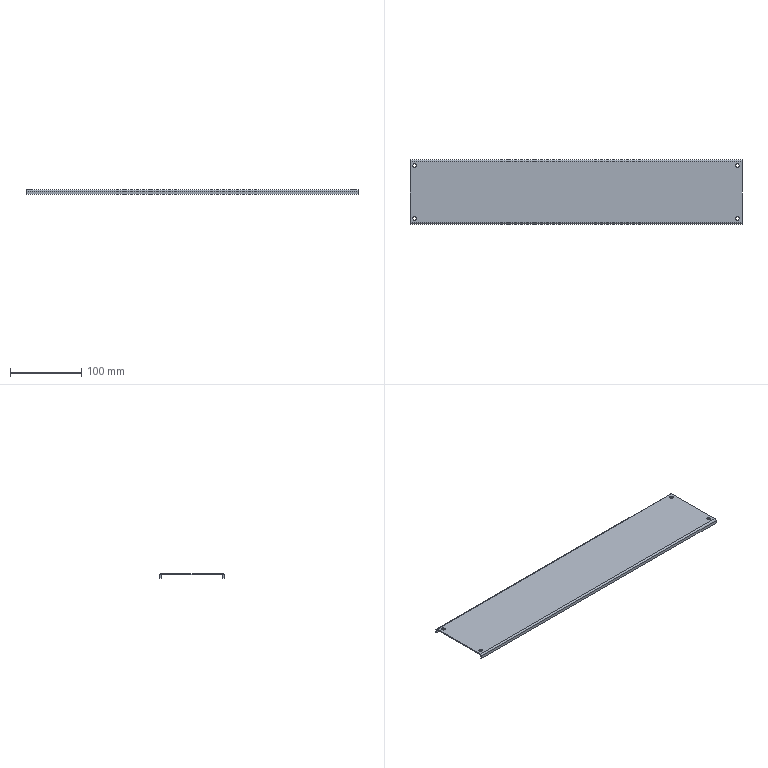Part | NX | features BREP 1 | 1 solid | 30 faces | box 466 x 90 x 6.5 mm | volume 68890 mm3 | plane 18 | cylinder 12 | commonest cylinder face diameters 5 x8 1.473 x2 4.473 x2
STEP:
#1=CARTESIAN_POINT('',(-229.,37.,-1.5));
#2=VERTEX_POINT('',#1);
#3=CARTESIAN_POINT('',(-224.,37.,-1.5));
#4=VERTEX_POINT('',#3);
#5=CARTESIAN_POINT('',(-226.5,37.,-1.5));
#6=DIRECTION('',(0.,0.,1.));
#7=DIRECTION('',(1.,0.,0.));
#8=AXIS2_PLACEMENT_3D('',#5,#6,#7);
#9=CIRCLE('',#8,2.5);
#10=EDGE_CURVE('',#2,#4,#9,.T.);
#11=ORIENTED_EDGE('',*,*,#10,.F.);
#12=CARTESIAN_POINT('',(-229.,37.,0.));
#13=VERTEX_POINT('',#12);
#14=CARTESIAN_POINT('',(-229.,37.,-10.));
#15=DIRECTION('',(0.,0.,1.));
#16=VECTOR('',#15,1000.);
#17=LINE('',#14,#16);
#18=EDGE_CURVE('',#13,#2,#17,.F.);
#19=ORIENTED_EDGE('',*,*,#18,.F.);
#20=CARTESIAN_POINT('',(-224.,37.,0.));
#21=VERTEX_POINT('',#20);
#22=CARTESIAN_POINT('',(-226.5,37.,0.));
#23=DIRECTION('',(0.,0.,1.));
#24=DIRECTION('',(-1.,0.,0.));
#25=AXIS2_PLACEMENT_3D('',#22,#23,#24);
#26=CIRCLE('',#25,2.5);
#27=EDGE_CURVE('',#13,#21,#26,.T.);
#28=ORIENTED_EDGE('',*,*,#27,.T.);
#29=CARTESIAN_POINT('',(-224.,37.,-10.));
#30=DIRECTION('',(0.,0.,1.));
#31=VECTOR('',#30,1000.);
#32=LINE('',#29,#31);
#33=EDGE_CURVE('',#21,#4,#32,.F.);
#34=ORIENTED_EDGE('',*,*,#33,.T.);
#35=EDGE_LOOP('',(#11,#19,#28,#34));
#36=FACE_BOUND('',#35,.T.);
#37=CARTESIAN_POINT('',(-226.5,37.,-10.));
#38=DIRECTION('',(0.,0.,1.));
#39=DIRECTION('',(1.,0.,0.));
#40=AXIS2_PLACEMENT_3D('',#37,#38,#39);
#41=CYLINDRICAL_SURFACE('',#40,2.5);
#42=ADVANCED_FACE('',(#36),#41,.F.);
#43=CARTESIAN_POINT('',(-229.,-37.,-1.5));
#44=VERTEX_POINT('',#43);
#45=CARTESIAN_POINT('',(-224.,-37.,-1.5));
#46=VERTEX_POINT('',#45);
#47=CARTESIAN_POINT('',(-226.5,-37.,-1.5));
#48=DIRECTION('',(0.,0.,1.));
#49=DIRECTION('',(1.,0.,0.));
#50=AXIS2_PLACEMENT_3D('',#47,#48,#49);
#51=CIRCLE('',#50,2.5);
#52=EDGE_CURVE('',#44,#46,#51,.T.);
#53=ORIENTED_EDGE('',*,*,#52,.F.);
#54=CARTESIAN_POINT('',(-229.,-37.,0.));
#55=VERTEX_POINT('',#54);
#56=CARTESIAN_POINT('',(-229.,-37.,-10.));
#57=DIRECTION('',(0.,0.,1.));
#58=VECTOR('',#57,1000.);
#59=LINE('',#56,#58);
#60=EDGE_CURVE('',#55,#44,#59,.F.);
#61=ORIENTED_EDGE('',*,*,#60,.F.);
#62=CARTESIAN_POINT('',(-224.,-37.,0.));
#63=VERTEX_POINT('',#62);
#64=CARTESIAN_POINT('',(-226.5,-37.,0.));
#65=DIRECTION('',(0.,0.,1.));
#66=DIRECTION('',(-1.,0.,0.));
#67=AXIS2_PLACEMENT_3D('',#64,#65,#66);
#68=CIRCLE('',#67,2.5);
#69=EDGE_CURVE('',#55,#63,#68,.T.);
#70=ORIENTED_EDGE('',*,*,#69,.T.);
#71=CARTESIAN_POINT('',(-224.,-37.,-10.));
#72=DIRECTION('',(0.,0.,1.));
#73=VECTOR('',#72,1000.);
#74=LINE('',#71,#73);
#75=EDGE_CURVE('',#63,#46,#74,.F.);
#76=ORIENTED_EDGE('',*,*,#75,.T.);
#77=EDGE_LOOP('',(#53,#61,#70,#76));
#78=FACE_BOUND('',#77,.T.);
#79=CARTESIAN_POINT('',(-226.5,-37.,-10.));
#80=DIRECTION('',(0.,0.,1.));
#81=DIRECTION('',(1.,0.,0.));
#82=AXIS2_PLACEMENT_3D('',#79,#80,#81);
#83=CYLINDRICAL_SURFACE('',#82,2.5);
#84=ADVANCED_FACE('',(#78),#83,.F.);
#85=CARTESIAN_POINT('',(224.,-37.,-1.5));
#86=VERTEX_POINT('',#85);
#87=CARTESIAN_POINT('',(229.,-37.,-1.5));
#88=VERTEX_POINT('',#87);
#89=CARTESIAN_POINT('',(226.5,-37.,-1.5));
#90=DIRECTION('',(0.,0.,1.));
#91=DIRECTION('',(1.,0.,0.));
#92=AXIS2_PLACEMENT_3D('',#89,#90,#91);
#93=CIRCLE('',#92,2.5);
#94=EDGE_CURVE('',#86,#88,#93,.T.);
#95=ORIENTED_EDGE('',*,*,#94,.F.);
#96=CARTESIAN_POINT('',(224.,-37.,0.));
#97=VERTEX_POINT('',#96);
#98=CARTESIAN_POINT('',(224.,-37.,-10.));
#99=DIRECTION('',(0.,0.,1.));
#100=VECTOR('',#99,1000.);
#101=LINE('',#98,#100);
#102=EDGE_CURVE('',#97,#86,#101,.F.);
#103=ORIENTED_EDGE('',*,*,#102,.F.);
#104=CARTESIAN_POINT('',(229.,-37.,0.));
#105=VERTEX_POINT('',#104);
#106=CARTESIAN_POINT('',(226.5,-37.,0.));
#107=DIRECTION('',(0.,0.,1.));
#108=DIRECTION('',(1.,0.,0.));
#109=AXIS2_PLACEMENT_3D('',#106,#107,#108);
#110=CIRCLE('',#109,2.5);
#111=EDGE_CURVE('',#97,#105,#110,.T.);
#112=ORIENTED_EDGE('',*,*,#111,.T.);
#113=CARTESIAN_POINT('',(229.,-37.,-10.));
#114=DIRECTION('',(0.,0.,1.));
#115=VECTOR('',#114,1000.);
#116=LINE('',#113,#115);
#117=EDGE_CURVE('',#105,#88,#116,.F.);
#118=ORIENTED_EDGE('',*,*,#117,.T.);
#119=EDGE_LOOP('',(#95,#103,#112,#118));
#120=FACE_BOUND('',#119,.T.);
#121=CARTESIAN_POINT('',(226.5,-37.,-10.));
#122=DIRECTION('',(0.,0.,1.));
#123=DIRECTION('',(1.,0.,0.));
#124=AXIS2_PLACEMENT_3D('',#121,#122,#123);
#125=CYLINDRICAL_SURFACE('',#124,2.5);
#126=ADVANCED_FACE('',(#120),#125,.F.);
#127=CARTESIAN_POINT('',(224.,37.,-1.5));
#128=VERTEX_POINT('',#127);
#129=CARTESIAN_POINT('',(229.,37.,-1.5));
#130=VERTEX_POINT('',#129);
#131=CARTESIAN_POINT('',(226.5,37.,-1.5));
#132=DIRECTION('',(0.,0.,1.));
#133=DIRECTION('',(1.,0.,0.));
#134=AXIS2_PLACEMENT_3D('',#131,#132,#133);
#135=CIRCLE('',#134,2.5);
#136=EDGE_CURVE('',#128,#130,#135,.T.);
#137=ORIENTED_EDGE('',*,*,#136,.F.);
#138=CARTESIAN_POINT('',(224.,37.,0.));
#139=VERTEX_POINT('',#138);
#140=CARTESIAN_POINT('',(224.,37.,-10.));
#141=DIRECTION('',(0.,0.,1.));
#142=VECTOR('',#141,1000.);
#143=LINE('',#140,#142);
#144=EDGE_CURVE('',#139,#128,#143,.F.);
#145=ORIENTED_EDGE('',*,*,#144,.F.);
#146=CARTESIAN_POINT('',(229.,37.,0.));
#147=VERTEX_POINT('',#146);
#148=CARTESIAN_POINT('',(226.5,37.,0.));
#149=DIRECTION('',(0.,0.,1.));
#150=DIRECTION('',(1.,0.,0.));
#151=AXIS2_PLACEMENT_3D('',#148,#149,#150);
#152=CIRCLE('',#151,2.5);
#153=EDGE_CURVE('',#139,#147,#152,.T.);
#154=ORIENTED_EDGE('',*,*,#153,.T.);
#155=CARTESIAN_POINT('',(229.,37.,-10.));
#156=DIRECTION('',(0.,0.,1.));
#157=VECTOR('',#156,1000.);
#158=LINE('',#155,#157);
#159=EDGE_CURVE('',#147,#130,#158,.F.);
#160=ORIENTED_EDGE('',*,*,#159,.T.);
#161=EDGE_LOOP('',(#137,#145,#154,#160));
#162=FACE_BOUND('',#161,.T.);
#163=CARTESIAN_POINT('',(226.5,37.,-10.));
#164=DIRECTION('',(0.,0.,1.));
#165=DIRECTION('',(1.,0.,0.));
#166=AXIS2_PLACEMENT_3D('',#163,#164,#165);
#167=CYLINDRICAL_SURFACE('',#166,2.5);
#168=ADVANCED_FACE('',(#162),#167,.F.);
#169=CARTESIAN_POINT('',(233.,42.763,-1.5));
#170=VERTEX_POINT('',#169);
#171=CARTESIAN_POINT('',(-233.,42.763,-1.5));
#172=VERTEX_POINT('',#171);
#173=CARTESIAN_POINT('',(233.,42.763,-1.5));
#174=DIRECTION('',(-1.,0.,0.));
#175=VECTOR('',#174,1000.);
#176=LINE('',#173,#175);
#177=EDGE_CURVE('',#170,#172,#176,.T.);
#178=ORIENTED_EDGE('',*,*,#177,.F.);
#179=CARTESIAN_POINT('',(233.,-42.763,-1.5));
#180=VERTEX_POINT('',#179);
#181=CARTESIAN_POINT('',(233.,43.5,-1.5));
#182=DIRECTION('',(0.,1.,0.));
#183=VECTOR('',#182,1000.);
#184=LINE('',#181,#183);
#185=EDGE_CURVE('',#180,#170,#184,.T.);
#186=ORIENTED_EDGE('',*,*,#185,.F.);
#187=CARTESIAN_POINT('',(-233.,-42.763,-1.5));
#188=VERTEX_POINT('',#187);
#189=CARTESIAN_POINT('',(-233.,-42.763,-1.5));
#190=DIRECTION('',(1.,0.,0.));
#191=VECTOR('',#190,1000.);
#192=LINE('',#189,#191);
#193=EDGE_CURVE('',#188,#180,#192,.T.);
#194=ORIENTED_EDGE('',*,*,#193,.F.);
#195=CARTESIAN_POINT('',(-233.,43.5,-1.5));
#196=DIRECTION('',(0.,-1.,0.));
#197=VECTOR('',#196,1000.);
#198=LINE('',#195,#197);
#199=EDGE_CURVE('',#172,#188,#198,.T.);
#200=ORIENTED_EDGE('',*,*,#199,.F.);
#201=EDGE_LOOP('',(#178,#186,#194,#200));
#202=FACE_BOUND('',#201,.T.);
#203=CARTESIAN_POINT('',(-226.5,37.,-1.5));
#204=DIRECTION('',(0.,0.,1.));
#205=DIRECTION('',(1.,0.,0.));
#206=AXIS2_PLACEMENT_3D('',#203,#204,#205);
#207=CIRCLE('',#206,2.5);
#208=EDGE_CURVE('',#4,#2,#207,.T.);
#209=ORIENTED_EDGE('',*,*,#208,.T.);
#210=ORIENTED_EDGE('',*,*,#10,.T.);
#211=EDGE_LOOP('',(#209,#210));
#212=FACE_BOUND('',#211,.T.);
#213=CARTESIAN_POINT('',(-226.5,-37.,-1.5));
#214=DIRECTION('',(0.,0.,1.));
#215=DIRECTION('',(1.,0.,0.));
#216=AXIS2_PLACEMENT_3D('',#213,#214,#215);
#217=CIRCLE('',#216,2.5);
#218=EDGE_CURVE('',#46,#44,#217,.T.);
#219=ORIENTED_EDGE('',*,*,#218,.T.);
#220=ORIENTED_EDGE('',*,*,#52,.T.);
#221=EDGE_LOOP('',(#219,#220));
#222=FACE_BOUND('',#221,.T.);
#223=CARTESIAN_POINT('',(226.5,-37.,-1.5));
#224=DIRECTION('',(0.,0.,1.));
#225=DIRECTION('',(1.,0.,0.));
#226=AXIS2_PLACEMENT_3D('',#223,#224,#225);
#227=CIRCLE('',#226,2.5);
#228=EDGE_CURVE('',#88,#86,#227,.T.);
#229=ORIENTED_EDGE('',*,*,#228,.T.);
#230=ORIENTED_EDGE('',*,*,#94,.T.);
#231=EDGE_LOOP('',(#229,#230));
#232=FACE_BOUND('',#231,.T.);
#233=CARTESIAN_POINT('',(226.5,37.,-1.5));
#234=DIRECTION('',(0.,0.,1.));
#235=DIRECTION('',(1.,0.,0.));
#236=AXIS2_PLACEMENT_3D('',#233,#234,#235);
#237=CIRCLE('',#236,2.5);
#238=EDGE_CURVE('',#130,#128,#237,.T.);
#239=ORIENTED_EDGE('',*,*,#238,.T.);
#240=ORIENTED_EDGE('',*,*,#136,.T.);
#241=EDGE_LOOP('',(#239,#240));
#242=FACE_BOUND('',#241,.T.);
#243=CARTESIAN_POINT('',(0.,0.,-1.5));
#244=DIRECTION('',(0.,0.,1.));
#245=DIRECTION('',(1.,0.,0.));
#246=AXIS2_PLACEMENT_3D('',#243,#244,#245);
#247=PLANE('',#246);
#248=ADVANCED_FACE('',(#202,#212,#222,#232,#242),#247,.F.);
#249=CARTESIAN_POINT('',(233.,-42.763,0.));
#250=VERTEX_POINT('',#249);
#251=CARTESIAN_POINT('',(233.,42.763,0.));
#252=VERTEX_POINT('',#251);
#253=CARTESIAN_POINT('',(233.,43.5,0.));
#254=DIRECTION('',(0.,1.,0.));
#255=VECTOR('',#254,1000.);
#256=LINE('',#253,#255);
#257=EDGE_CURVE('',#250,#252,#256,.T.);
#258=ORIENTED_EDGE('',*,*,#257,.T.);
#259=CARTESIAN_POINT('',(-233.,42.763,0.));
#260=VERTEX_POINT('',#259);
#261=CARTESIAN_POINT('',(233.,42.763,0.));
#262=DIRECTION('',(-1.,0.,0.));
#263=VECTOR('',#262,1000.);
#264=LINE('',#261,#263);
#265=EDGE_CURVE('',#252,#260,#264,.T.);
#266=ORIENTED_EDGE('',*,*,#265,.T.);
#267=CARTESIAN_POINT('',(-233.,-42.763,0.));
#268=VERTEX_POINT('',#267);
#269=CARTESIAN_POINT('',(-233.,43.5,0.));
#270=DIRECTION('',(0.,-1.,0.));
#271=VECTOR('',#270,1000.);
#272=LINE('',#269,#271);
#273=EDGE_CURVE('',#260,#268,#272,.T.);
#274=ORIENTED_EDGE('',*,*,#273,.T.);
#275=CARTESIAN_POINT('',(-233.,-42.763,0.));
#276=DIRECTION('',(1.,0.,0.));
#277=VECTOR('',#276,1000.);
#278=LINE('',#275,#277);
#279=EDGE_CURVE('',#268,#250,#278,.T.);
#280=ORIENTED_EDGE('',*,*,#279,.T.);
#281=EDGE_LOOP('',(#258,#266,#274,#280));
#282=FACE_BOUND('',#281,.T.);
#283=CARTESIAN_POINT('',(-226.5,37.,0.));
#284=DIRECTION('',(0.,0.,1.));
#285=DIRECTION('',(-1.,0.,0.));
#286=AXIS2_PLACEMENT_3D('',#283,#284,#285);
#287=CIRCLE('',#286,2.5);
#288=EDGE_CURVE('',#21,#13,#287,.T.);
#289=ORIENTED_EDGE('',*,*,#288,.F.);
#290=ORIENTED_EDGE('',*,*,#27,.F.);
#291=EDGE_LOOP('',(#289,#290));
#292=FACE_BOUND('',#291,.T.);
#293=CARTESIAN_POINT('',(-226.5,-37.,0.));
#294=DIRECTION('',(0.,0.,1.));
#295=DIRECTION('',(-1.,0.,0.));
#296=AXIS2_PLACEMENT_3D('',#293,#294,#295);
#297=CIRCLE('',#296,2.5);
#298=EDGE_CURVE('',#63,#55,#297,.T.);
#299=ORIENTED_EDGE('',*,*,#298,.F.);
#300=ORIENTED_EDGE('',*,*,#69,.F.);
#301=EDGE_LOOP('',(#299,#300));
#302=FACE_BOUND('',#301,.T.);
#303=CARTESIAN_POINT('',(226.5,-37.,0.));
#304=DIRECTION('',(0.,0.,1.));
#305=DIRECTION('',(1.,0.,0.));
#306=AXIS2_PLACEMENT_3D('',#303,#304,#305);
#307=CIRCLE('',#306,2.5);
#308=EDGE_CURVE('',#105,#97,#307,.T.);
#309=ORIENTED_EDGE('',*,*,#308,.F.);
#310=ORIENTED_EDGE('',*,*,#111,.F.);
#311=EDGE_LOOP('',(#309,#310));
#312=FACE_BOUND('',#311,.T.);
#313=CARTESIAN_POINT('',(226.5,37.,0.));
#314=DIRECTION('',(0.,0.,1.));
#315=DIRECTION('',(1.,0.,0.));
#316=AXIS2_PLACEMENT_3D('',#313,#314,#315);
#317=CIRCLE('',#316,2.5);
#318=EDGE_CURVE('',#147,#139,#317,.T.);
#319=ORIENTED_EDGE('',*,*,#318,.F.);
#320=ORIENTED_EDGE('',*,*,#153,.F.);
#321=EDGE_LOOP('',(#319,#320));
#322=FACE_BOUND('',#321,.T.);
#323=CARTESIAN_POINT('',(0.,0.,0.));
#324=DIRECTION('',(0.,0.,1.));
#325=DIRECTION('',(1.,0.,0.));
#326=AXIS2_PLACEMENT_3D('',#323,#324,#325);
#327=PLANE('',#326);
#328=ADVANCED_FACE('',(#282,#292,#302,#312,#322),#327,.T.);
#329=ORIENTED_EDGE('',*,*,#185,.T.);
#330=CARTESIAN_POINT('',(233.,42.763,-1.5));
#331=DIRECTION('',(0.,0.,1.));
#332=VECTOR('',#331,1000.);
#333=LINE('',#330,#332);
#334=EDGE_CURVE('',#170,#252,#333,.T.);
#335=ORIENTED_EDGE('',*,*,#334,.T.);
#336=ORIENTED_EDGE('',*,*,#257,.F.);
#337=CARTESIAN_POINT('',(233.,-42.763,-1.5));
#338=DIRECTION('',(0.,0.,1.));
#339=VECTOR('',#338,1000.);
#340=LINE('',#337,#339);
#341=EDGE_CURVE('',#180,#250,#340,.T.);
#342=ORIENTED_EDGE('',*,*,#341,.F.);
#343=EDGE_LOOP('',(#329,#335,#336,#342));
#344=FACE_BOUND('',#343,.T.);
#345=CARTESIAN_POINT('',(233.,43.5,-1.5));
#346=DIRECTION('',(1.,0.,0.));
#347=DIRECTION('',(0.,1.,0.));
#348=AXIS2_PLACEMENT_3D('',#345,#346,#347);
#349=PLANE('',#348);
#350=ADVANCED_FACE('',(#344),#349,.T.);
#351=CARTESIAN_POINT('',(-233.,42.763,-1.5));
#352=DIRECTION('',(0.,0.,1.));
#353=VECTOR('',#352,1000.);
#354=LINE('',#351,#353);
#355=EDGE_CURVE('',#172,#260,#354,.T.);
#356=ORIENTED_EDGE('',*,*,#355,.F.);
#357=ORIENTED_EDGE('',*,*,#199,.T.);
#358=CARTESIAN_POINT('',(-233.,-42.763,-1.5));
#359=DIRECTION('',(0.,0.,1.));
#360=VECTOR('',#359,1000.);
#361=LINE('',#358,#360);
#362=EDGE_CURVE('',#188,#268,#361,.T.);
#363=ORIENTED_EDGE('',*,*,#362,.T.);
#364=ORIENTED_EDGE('',*,*,#273,.F.);
#365=EDGE_LOOP('',(#356,#357,#363,#364));
#366=FACE_BOUND('',#365,.T.);
#367=CARTESIAN_POINT('',(-233.,43.5,-1.5));
#368=DIRECTION('',(-1.,0.,0.));
#369=DIRECTION('',(0.,0.,1.));
#370=AXIS2_PLACEMENT_3D('',#367,#368,#369);
#371=PLANE('',#370);
#372=ADVANCED_FACE('',(#366),#371,.T.);
#373=CARTESIAN_POINT('',(233.,-43.5,-2.237));
#374=VERTEX_POINT('',#373);
#375=CARTESIAN_POINT('',(233.,-45.,-2.237));
#376=VERTEX_POINT('',#375);
#377=CARTESIAN_POINT('',(233.,-43.5,-2.237));
#378=DIRECTION('',(0.,-1.,0.));
#379=VECTOR('',#378,1000.);
#380=LINE('',#377,#379);
#381=EDGE_CURVE('',#374,#376,#380,.T.);
#382=ORIENTED_EDGE('',*,*,#381,.F.);
#383=CARTESIAN_POINT('',(233.,-42.763,-2.237));
#384=DIRECTION('',(1.,0.,0.));
#385=DIRECTION('',(0.,0.,1.));
#386=AXIS2_PLACEMENT_3D('',#383,#384,#385);
#387=CIRCLE('',#386,0.7366);
#388=EDGE_CURVE('',#180,#374,#387,.T.);
#389=ORIENTED_EDGE('',*,*,#388,.F.);
#390=ORIENTED_EDGE('',*,*,#341,.T.);
#391=CARTESIAN_POINT('',(233.,-42.763,-2.237));
#392=DIRECTION('',(1.,0.,0.));
#393=DIRECTION('',(0.,0.,1.));
#394=AXIS2_PLACEMENT_3D('',#391,#392,#393);
#395=CIRCLE('',#394,2.237);
#396=EDGE_CURVE('',#250,#376,#395,.T.);
#397=ORIENTED_EDGE('',*,*,#396,.T.);
#398=EDGE_LOOP('',(#382,#389,#390,#397));
#399=FACE_BOUND('',#398,.T.);
#400=CARTESIAN_POINT('',(233.,-42.763,-2.237));
#401=DIRECTION('',(1.,0.,0.));
#402=DIRECTION('',(0.,1.,0.));
#403=AXIS2_PLACEMENT_3D('',#400,#401,#402);
#404=PLANE('',#403);
#405=ADVANCED_FACE('',(#399),#404,.T.);
#406=CARTESIAN_POINT('',(-233.,-43.5,-2.237));
#407=VERTEX_POINT('',#406);
#408=CARTESIAN_POINT('',(-233.,-42.763,-2.237));
#409=DIRECTION('',(-1.,0.,0.));
#410=DIRECTION('',(0.,0.,1.));
#411=AXIS2_PLACEMENT_3D('',#408,#409,#410);
#412=CIRCLE('',#411,0.7366);
#413=EDGE_CURVE('',#407,#188,#412,.T.);
#414=ORIENTED_EDGE('',*,*,#413,.F.);
#415=CARTESIAN_POINT('',(-233.,-45.,-2.237));
#416=VERTEX_POINT('',#415);
#417=CARTESIAN_POINT('',(-233.,-43.5,-2.237));
#418=DIRECTION('',(0.,-1.,0.));
#419=VECTOR('',#418,1000.);
#420=LINE('',#417,#419);
#421=EDGE_CURVE('',#407,#416,#420,.T.);
#422=ORIENTED_EDGE('',*,*,#421,.T.);
#423=CARTESIAN_POINT('',(-233.,-42.763,-2.237));
#424=DIRECTION('',(-1.,0.,0.));
#425=DIRECTION('',(0.,0.,1.));
#426=AXIS2_PLACEMENT_3D('',#423,#424,#425);
#427=CIRCLE('',#426,2.237);
#428=EDGE_CURVE('',#416,#268,#427,.T.);
#429=ORIENTED_EDGE('',*,*,#428,.T.);
#430=ORIENTED_EDGE('',*,*,#362,.F.);
#431=EDGE_LOOP('',(#414,#422,#429,#430));
#432=FACE_BOUND('',#431,.T.);
#433=CARTESIAN_POINT('',(-233.,-42.763,-2.237));
#434=DIRECTION('',(1.,0.,0.));
#435=DIRECTION('',(0.,1.,0.));
#436=AXIS2_PLACEMENT_3D('',#433,#434,#435);
#437=PLANE('',#436);
#438=ADVANCED_FACE('',(#432),#437,.F.);
#439=ORIENTED_EDGE('',*,*,#279,.F.);
#440=ORIENTED_EDGE('',*,*,#428,.F.);
#441=CARTESIAN_POINT('',(0.,-45.,-2.237));
#442=DIRECTION('',(-1.,0.,0.));
#443=VECTOR('',#442,1000.);
#444=LINE('',#441,#443);
#445=EDGE_CURVE('',#376,#416,#444,.T.);
#446=ORIENTED_EDGE('',*,*,#445,.F.);
#447=ORIENTED_EDGE('',*,*,#396,.F.);
#448=EDGE_LOOP('',(#439,#440,#446,#447));
#449=FACE_BOUND('',#448,.T.);
#450=CARTESIAN_POINT('',(-233.,-42.763,-2.237));
#451=DIRECTION('',(-1.,0.,0.));
#452=DIRECTION('',(0.,-1.,0.));
#453=AXIS2_PLACEMENT_3D('',#450,#451,#452);
#454=CYLINDRICAL_SURFACE('',#453,2.237);
#455=ADVANCED_FACE('',(#449),#454,.T.);
#456=ORIENTED_EDGE('',*,*,#193,.T.);
#457=ORIENTED_EDGE('',*,*,#388,.T.);
#458=CARTESIAN_POINT('',(233.,-43.5,-2.237));
#459=DIRECTION('',(-1.,0.,0.));
#460=VECTOR('',#459,1000.);
#461=LINE('',#458,#460);
#462=EDGE_CURVE('',#374,#407,#461,.T.);
#463=ORIENTED_EDGE('',*,*,#462,.T.);
#464=ORIENTED_EDGE('',*,*,#413,.T.);
#465=EDGE_LOOP('',(#456,#457,#463,#464));
#466=FACE_BOUND('',#465,.T.);
#467=CARTESIAN_POINT('',(-233.,-42.763,-2.237));
#468=DIRECTION('',(-1.,0.,0.));
#469=DIRECTION('',(0.,-1.,0.));
#470=AXIS2_PLACEMENT_3D('',#467,#468,#469);
#471=CYLINDRICAL_SURFACE('',#470,0.7366);
#472=ADVANCED_FACE('',(#466),#471,.F.);
#473=CARTESIAN_POINT('',(-233.,-45.,-6.5));
#474=VERTEX_POINT('',#473);
#475=CARTESIAN_POINT('',(-233.,-45.,-1.5));
#476=DIRECTION('',(0.,0.,1.));
#477=VECTOR('',#476,1000.);
#478=LINE('',#475,#477);
#479=EDGE_CURVE('',#474,#416,#478,.T.);
#480=ORIENTED_EDGE('',*,*,#479,.T.);
#481=ORIENTED_EDGE('',*,*,#421,.F.);
#482=CARTESIAN_POINT('',(-233.,-43.5,-6.5));
#483=VERTEX_POINT('',#482);
#484=CARTESIAN_POINT('',(-233.,-43.5,-1.5));
#485=DIRECTION('',(0.,0.,1.));
#486=VECTOR('',#485,1000.);
#487=LINE('',#484,#486);
#488=EDGE_CURVE('',#483,#407,#487,.T.);
#489=ORIENTED_EDGE('',*,*,#488,.F.);
#490=CARTESIAN_POINT('',(-233.,-45.,-6.5));
#491=DIRECTION('',(0.,1.,0.));
#492=VECTOR('',#491,1000.);
#493=LINE('',#490,#492);
#494=EDGE_CURVE('',#474,#483,#493,.T.);
#495=ORIENTED_EDGE('',*,*,#494,.F.);
#496=EDGE_LOOP('',(#480,#481,#489,#495));
#497=FACE_BOUND('',#496,.T.);
#498=CARTESIAN_POINT('',(-233.,-45.,-1.5));
#499=DIRECTION('',(-1.,0.,0.));
#500=DIRECTION('',(0.,1.,0.));
#501=AXIS2_PLACEMENT_3D('',#498,#499,#500);
#502=PLANE('',#501);
#503=ADVANCED_FACE('',(#497),#502,.T.);
#504=CARTESIAN_POINT('',(233.,-43.5,-6.5));
#505=VERTEX_POINT('',#504);
#506=CARTESIAN_POINT('',(233.,-43.5,-6.5));
#507=DIRECTION('',(0.,0.,-1.));
#508=VECTOR('',#507,1000.);
#509=LINE('',#506,#508);
#510=EDGE_CURVE('',#374,#505,#509,.T.);
#511=ORIENTED_EDGE('',*,*,#510,.F.);
#512=ORIENTED_EDGE('',*,*,#381,.T.);
#513=CARTESIAN_POINT('',(233.,-45.,-6.5));
#514=VERTEX_POINT('',#513);
#515=CARTESIAN_POINT('',(233.,-45.,-6.5));
#516=DIRECTION('',(0.,0.,-1.));
#517=VECTOR('',#516,1000.);
#518=LINE('',#515,#517);
#519=EDGE_CURVE('',#376,#514,#518,.T.);
#520=ORIENTED_EDGE('',*,*,#519,.T.);
#521=CARTESIAN_POINT('',(233.,-45.,-6.5));
#522=DIRECTION('',(0.,1.,0.));
#523=VECTOR('',#522,1000.);
#524=LINE('',#521,#523);
#525=EDGE_CURVE('',#514,#505,#524,.T.);
#526=ORIENTED_EDGE('',*,*,#525,.T.);
#527=EDGE_LOOP('',(#511,#512,#520,#526));
#528=FACE_BOUND('',#527,.T.);
#529=CARTESIAN_POINT('',(233.,-45.,-6.5));
#530=DIRECTION('',(1.,0.,0.));
#531=DIRECTION('',(0.,0.,-1.));
#532=AXIS2_PLACEMENT_3D('',#529,#530,#531);
#533=PLANE('',#532);
#534=ADVANCED_FACE('',(#528),#533,.T.);
#535=ORIENTED_EDGE('',*,*,#519,.F.);
#536=ORIENTED_EDGE('',*,*,#445,.T.);
#537=ORIENTED_EDGE('',*,*,#479,.F.);
#538=CARTESIAN_POINT('',(-233.,-45.,-6.5));
#539=DIRECTION('',(-1.,0.,0.));
#540=VECTOR('',#539,1000.);
#541=LINE('',#538,#540);
#542=EDGE_CURVE('',#514,#474,#541,.T.);
#543=ORIENTED_EDGE('',*,*,#542,.F.);
#544=EDGE_LOOP('',(#535,#536,#537,#543));
#545=FACE_BOUND('',#544,.T.);
#546=CARTESIAN_POINT('',(0.,-45.,0.));
#547=DIRECTION('',(0.,-1.,0.));
#548=DIRECTION('',(-1.,0.,0.));
#549=AXIS2_PLACEMENT_3D('',#546,#547,#548);
#550=PLANE('',#549);
#551=ADVANCED_FACE('',(#545),#550,.T.);
#552=ORIENTED_EDGE('',*,*,#462,.F.);
#553=ORIENTED_EDGE('',*,*,#510,.T.);
#554=CARTESIAN_POINT('',(-233.,-43.5,-6.5));
#555=DIRECTION('',(-1.,0.,0.));
#556=VECTOR('',#555,1000.);
#557=LINE('',#554,#556);
#558=EDGE_CURVE('',#505,#483,#557,.T.);
#559=ORIENTED_EDGE('',*,*,#558,.T.);
#560=ORIENTED_EDGE('',*,*,#488,.T.);
#561=EDGE_LOOP('',(#552,#553,#559,#560));
#562=FACE_BOUND('',#561,.T.);
#563=CARTESIAN_POINT('',(0.,-43.5,0.));
#564=DIRECTION('',(0.,-1.,0.));
#565=DIRECTION('',(-1.,0.,0.));
#566=AXIS2_PLACEMENT_3D('',#563,#564,#565);
#567=PLANE('',#566);
#568=ADVANCED_FACE('',(#562),#567,.F.);
#569=ORIENTED_EDGE('',*,*,#558,.F.);
#570=ORIENTED_EDGE('',*,*,#525,.F.);
#571=ORIENTED_EDGE('',*,*,#542,.T.);
#572=ORIENTED_EDGE('',*,*,#494,.T.);
#573=EDGE_LOOP('',(#569,#570,#571,#572));
#574=FACE_BOUND('',#573,.T.);
#575=CARTESIAN_POINT('',(-233.,-45.,-6.5));
#576=DIRECTION('',(0.,0.,-1.));
#577=DIRECTION('',(0.,-1.,0.));
#578=AXIS2_PLACEMENT_3D('',#575,#576,#577);
#579=PLANE('',#578);
#580=ADVANCED_FACE('',(#574),#579,.T.);
#581=CARTESIAN_POINT('',(-233.,43.5,-2.237));
#582=VERTEX_POINT('',#581);
#583=CARTESIAN_POINT('',(-233.,45.,-2.237));
#584=VERTEX_POINT('',#583);
#585=CARTESIAN_POINT('',(-233.,43.5,-2.237));
#586=DIRECTION('',(0.,1.,0.));
#587=VECTOR('',#586,1000.);
#588=LINE('',#585,#587);
#589=EDGE_CURVE('',#582,#584,#588,.T.);
#590=ORIENTED_EDGE('',*,*,#589,.F.);
#591=CARTESIAN_POINT('',(-233.,42.763,-2.237));
#592=DIRECTION('',(-1.,0.,0.));
#593=DIRECTION('',(0.,0.,-1.));
#594=AXIS2_PLACEMENT_3D('',#591,#592,#593);
#595=CIRCLE('',#594,0.7366);
#596=EDGE_CURVE('',#172,#582,#595,.T.);
#597=ORIENTED_EDGE('',*,*,#596,.F.);
#598=ORIENTED_EDGE('',*,*,#355,.T.);
#599=CARTESIAN_POINT('',(-233.,42.763,-2.237));
#600=DIRECTION('',(-1.,0.,0.));
#601=DIRECTION('',(0.,0.,-1.));
#602=AXIS2_PLACEMENT_3D('',#599,#600,#601);
#603=CIRCLE('',#602,2.237);
#604=EDGE_CURVE('',#260,#584,#603,.T.);
#605=ORIENTED_EDGE('',*,*,#604,.T.);
#606=EDGE_LOOP('',(#590,#597,#598,#605));
#607=FACE_BOUND('',#606,.T.);
#608=CARTESIAN_POINT('',(-233.,42.763,-2.237));
#609=DIRECTION('',(-1.,0.,0.));
#610=DIRECTION('',(0.,0.,1.));
#611=AXIS2_PLACEMENT_3D('',#608,#609,#610);
#612=PLANE('',#611);
#613=ADVANCED_FACE('',(#607),#612,.T.);
#614=CARTESIAN_POINT('',(233.,43.5,-2.237));
#615=VERTEX_POINT('',#614);
#616=CARTESIAN_POINT('',(233.,42.763,-2.237));
#617=DIRECTION('',(1.,0.,0.));
#618=DIRECTION('',(0.,0.,-1.));
#619=AXIS2_PLACEMENT_3D('',#616,#617,#618);
#620=CIRCLE('',#619,0.7366);
#621=EDGE_CURVE('',#615,#170,#620,.T.);
#622=ORIENTED_EDGE('',*,*,#621,.F.);
#623=CARTESIAN_POINT('',(233.,45.,-2.237));
#624=VERTEX_POINT('',#623);
#625=CARTESIAN_POINT('',(233.,43.5,-2.237));
#626=DIRECTION('',(0.,1.,0.));
#627=VECTOR('',#626,1000.);
#628=LINE('',#625,#627);
#629=EDGE_CURVE('',#615,#624,#628,.T.);
#630=ORIENTED_EDGE('',*,*,#629,.T.);
#631=CARTESIAN_POINT('',(233.,42.763,-2.237));
#632=DIRECTION('',(1.,0.,0.));
#633=DIRECTION('',(0.,0.,-1.));
#634=AXIS2_PLACEMENT_3D('',#631,#632,#633);
#635=CIRCLE('',#634,2.237);
#636=EDGE_CURVE('',#624,#252,#635,.T.);
#637=ORIENTED_EDGE('',*,*,#636,.T.);
#638=ORIENTED_EDGE('',*,*,#334,.F.);
#639=EDGE_LOOP('',(#622,#630,#637,#638));
#640=FACE_BOUND('',#639,.T.);
#641=CARTESIAN_POINT('',(233.,42.763,-2.237));
#642=DIRECTION('',(-1.,0.,0.));
#643=DIRECTION('',(0.,0.,1.));
#644=AXIS2_PLACEMENT_3D('',#641,#642,#643);
#645=PLANE('',#644);
#646=ADVANCED_FACE('',(#640),#645,.F.);
#647=ORIENTED_EDGE('',*,*,#265,.F.);
#648=ORIENTED_EDGE('',*,*,#636,.F.);
#649=CARTESIAN_POINT('',(0.,45.,-2.237));
#650=DIRECTION('',(-1.,0.,0.));
#651=VECTOR('',#650,1000.);
#652=LINE('',#649,#651);
#653=EDGE_CURVE('',#624,#584,#652,.T.);
#654=ORIENTED_EDGE('',*,*,#653,.T.);
#655=ORIENTED_EDGE('',*,*,#604,.F.);
#656=EDGE_LOOP('',(#647,#648,#654,#655));
#657=FACE_BOUND('',#656,.T.);
#658=CARTESIAN_POINT('',(233.,42.763,-2.237));
#659=DIRECTION('',(1.,0.,0.));
#660=DIRECTION('',(0.,1.,0.));
#661=AXIS2_PLACEMENT_3D('',#658,#659,#660);
#662=CYLINDRICAL_SURFACE('',#661,2.237);
#663=ADVANCED_FACE('',(#657),#662,.T.);
#664=ORIENTED_EDGE('',*,*,#177,.T.);
#665=ORIENTED_EDGE('',*,*,#596,.T.);
#666=CARTESIAN_POINT('',(-233.,43.5,-2.237));
#667=DIRECTION('',(1.,0.,0.));
#668=VECTOR('',#667,1000.);
#669=LINE('',#666,#668);
#670=EDGE_CURVE('',#582,#615,#669,.T.);
#671=ORIENTED_EDGE('',*,*,#670,.T.);
#672=ORIENTED_EDGE('',*,*,#621,.T.);
#673=EDGE_LOOP('',(#664,#665,#671,#672));
#674=FACE_BOUND('',#673,.T.);
#675=CARTESIAN_POINT('',(233.,42.763,-2.237));
#676=DIRECTION('',(1.,0.,0.));
#677=DIRECTION('',(0.,1.,0.));
#678=AXIS2_PLACEMENT_3D('',#675,#676,#677);
#679=CYLINDRICAL_SURFACE('',#678,0.7366);
#680=ADVANCED_FACE('',(#674),#679,.F.);
#681=CARTESIAN_POINT('',(-233.,43.5,-6.5));
#682=VERTEX_POINT('',#681);
#683=CARTESIAN_POINT('',(-233.,43.5,-1.5));
#684=DIRECTION('',(0.,0.,-1.));
#685=VECTOR('',#684,1000.);
#686=LINE('',#683,#685);
#687=EDGE_CURVE('',#582,#682,#686,.T.);
#688=ORIENTED_EDGE('',*,*,#687,.F.);
#689=ORIENTED_EDGE('',*,*,#589,.T.);
#690=CARTESIAN_POINT('',(-233.,45.,-6.5));
#691=VERTEX_POINT('',#690);
#692=CARTESIAN_POINT('',(-233.,45.,-1.5));
#693=DIRECTION('',(0.,0.,-1.));
#694=VECTOR('',#693,1000.);
#695=LINE('',#692,#694);
#696=EDGE_CURVE('',#584,#691,#695,.T.);
#697=ORIENTED_EDGE('',*,*,#696,.T.);
#698=CARTESIAN_POINT('',(-233.,45.,-6.5));
#699=DIRECTION('',(0.,-1.,0.));
#700=VECTOR('',#699,1000.);
#701=LINE('',#698,#700);
#702=EDGE_CURVE('',#691,#682,#701,.T.);
#703=ORIENTED_EDGE('',*,*,#702,.T.);
#704=EDGE_LOOP('',(#688,#689,#697,#703));
#705=FACE_BOUND('',#704,.T.);
#706=CARTESIAN_POINT('',(-233.,45.,-1.5));
#707=DIRECTION('',(-1.,0.,0.));
#708=DIRECTION('',(0.,1.,0.));
#709=AXIS2_PLACEMENT_3D('',#706,#707,#708);
#710=PLANE('',#709);
#711=ADVANCED_FACE('',(#705),#710,.T.);
#712=CARTESIAN_POINT('',(233.,45.,-6.5));
#713=VERTEX_POINT('',#712);
#714=CARTESIAN_POINT('',(233.,45.,-6.5));
#715=DIRECTION('',(0.,0.,1.));
#716=VECTOR('',#715,1000.);
#717=LINE('',#714,#716);
#718=EDGE_CURVE('',#713,#624,#717,.T.);
#719=ORIENTED_EDGE('',*,*,#718,.T.);
#720=ORIENTED_EDGE('',*,*,#629,.F.);
#721=CARTESIAN_POINT('',(233.,43.5,-6.5));
#722=VERTEX_POINT('',#721);
#723=CARTESIAN_POINT('',(233.,43.5,-6.5));
#724=DIRECTION('',(0.,0.,1.));
#725=VECTOR('',#724,1000.);
#726=LINE('',#723,#725);
#727=EDGE_CURVE('',#722,#615,#726,.T.);
#728=ORIENTED_EDGE('',*,*,#727,.F.);
#729=CARTESIAN_POINT('',(233.,45.,-6.5));
#730=DIRECTION('',(0.,-1.,0.));
#731=VECTOR('',#730,1000.);
#732=LINE('',#729,#731);
#733=EDGE_CURVE('',#713,#722,#732,.T.);
#734=ORIENTED_EDGE('',*,*,#733,.F.);
#735=EDGE_LOOP('',(#719,#720,#728,#734));
#736=FACE_BOUND('',#735,.T.);
#737=CARTESIAN_POINT('',(233.,45.,-6.5));
#738=DIRECTION('',(1.,0.,0.));
#739=DIRECTION('',(0.,0.,-1.));
#740=AXIS2_PLACEMENT_3D('',#737,#738,#739);
#741=PLANE('',#740);
#742=ADVANCED_FACE('',(#736),#741,.T.);
#743=ORIENTED_EDGE('',*,*,#653,.F.);
#744=ORIENTED_EDGE('',*,*,#718,.F.);
#745=CARTESIAN_POINT('',(-233.,45.,-6.5));
#746=DIRECTION('',(1.,0.,0.));
#747=VECTOR('',#746,1000.);
#748=LINE('',#745,#747);
#749=EDGE_CURVE('',#691,#713,#748,.T.);
#750=ORIENTED_EDGE('',*,*,#749,.F.);
#751=ORIENTED_EDGE('',*,*,#696,.F.);
#752=EDGE_LOOP('',(#743,#744,#750,#751));
#753=FACE_BOUND('',#752,.T.);
#754=CARTESIAN_POINT('',(0.,45.,0.));
#755=DIRECTION('',(0.,-1.,0.));
#756=DIRECTION('',(0.,0.,-1.));
#757=AXIS2_PLACEMENT_3D('',#754,#755,#756);
#758=PLANE('',#757);
#759=ADVANCED_FACE('',(#753),#758,.F.);
#760=ORIENTED_EDGE('',*,*,#727,.T.);
#761=ORIENTED_EDGE('',*,*,#670,.F.);
#762=ORIENTED_EDGE('',*,*,#687,.T.);
#763=CARTESIAN_POINT('',(-233.,43.5,-6.5));
#764=DIRECTION('',(1.,0.,0.));
#765=VECTOR('',#764,1000.);
#766=LINE('',#763,#765);
#767=EDGE_CURVE('',#682,#722,#766,.T.);
#768=ORIENTED_EDGE('',*,*,#767,.T.);
#769=EDGE_LOOP('',(#760,#761,#762,#768));
#770=FACE_BOUND('',#769,.T.);
#771=CARTESIAN_POINT('',(0.,43.5,0.));
#772=DIRECTION('',(0.,-1.,0.));
#773=DIRECTION('',(0.,0.,-1.));
#774=AXIS2_PLACEMENT_3D('',#771,#772,#773);
#775=PLANE('',#774);
#776=ADVANCED_FACE('',(#770),#775,.T.);
#777=ORIENTED_EDGE('',*,*,#767,.F.);
#778=ORIENTED_EDGE('',*,*,#702,.F.);
#779=ORIENTED_EDGE('',*,*,#749,.T.);
#780=ORIENTED_EDGE('',*,*,#733,.T.);
#781=EDGE_LOOP('',(#777,#778,#779,#780));
#782=FACE_BOUND('',#781,.T.);
#783=CARTESIAN_POINT('',(-233.,45.,-6.5));
#784=DIRECTION('',(0.,0.,-1.));
#785=DIRECTION('',(-1.,0.,0.));
#786=AXIS2_PLACEMENT_3D('',#783,#784,#785);
#787=PLANE('',#786);
#788=ADVANCED_FACE('',(#782),#787,.T.);
#789=ORIENTED_EDGE('',*,*,#144,.T.);
#790=ORIENTED_EDGE('',*,*,#238,.F.);
#791=ORIENTED_EDGE('',*,*,#159,.F.);
#792=ORIENTED_EDGE('',*,*,#318,.T.);
#793=EDGE_LOOP('',(#789,#790,#791,#792));
#794=FACE_BOUND('',#793,.T.);
#795=CARTESIAN_POINT('',(226.5,37.,-10.));
#796=DIRECTION('',(0.,0.,1.));
#797=DIRECTION('',(1.,0.,0.));
#798=AXIS2_PLACEMENT_3D('',#795,#796,#797);
#799=CYLINDRICAL_SURFACE('',#798,2.5);
#800=ADVANCED_FACE('',(#794),#799,.F.);
#801=ORIENTED_EDGE('',*,*,#102,.T.);
#802=ORIENTED_EDGE('',*,*,#228,.F.);
#803=ORIENTED_EDGE('',*,*,#117,.F.);
#804=ORIENTED_EDGE('',*,*,#308,.T.);
#805=EDGE_LOOP('',(#801,#802,#803,#804));
#806=FACE_BOUND('',#805,.T.);
#807=CARTESIAN_POINT('',(226.5,-37.,-10.));
#808=DIRECTION('',(0.,0.,1.));
#809=DIRECTION('',(1.,0.,0.));
#810=AXIS2_PLACEMENT_3D('',#807,#808,#809);
#811=CYLINDRICAL_SURFACE('',#810,2.5);
#812=ADVANCED_FACE('',(#806),#811,.F.);
#813=ORIENTED_EDGE('',*,*,#60,.T.);
#814=ORIENTED_EDGE('',*,*,#218,.F.);
#815=ORIENTED_EDGE('',*,*,#75,.F.);
#816=ORIENTED_EDGE('',*,*,#298,.T.);
#817=EDGE_LOOP('',(#813,#814,#815,#816));
#818=FACE_BOUND('',#817,.T.);
#819=CARTESIAN_POINT('',(-226.5,-37.,-10.));
#820=DIRECTION('',(0.,0.,1.));
#821=DIRECTION('',(1.,0.,0.));
#822=AXIS2_PLACEMENT_3D('',#819,#820,#821);
#823=CYLINDRICAL_SURFACE('',#822,2.5);
#824=ADVANCED_FACE('',(#818),#823,.F.);
#825=ORIENTED_EDGE('',*,*,#18,.T.);
#826=ORIENTED_EDGE('',*,*,#208,.F.);
#827=ORIENTED_EDGE('',*,*,#33,.F.);
#828=ORIENTED_EDGE('',*,*,#288,.T.);
#829=EDGE_LOOP('',(#825,#826,#827,#828));
#830=FACE_BOUND('',#829,.T.);
#831=CARTESIAN_POINT('',(-226.5,37.,-10.));
#832=DIRECTION('',(0.,0.,1.));
#833=DIRECTION('',(1.,0.,0.));
#834=AXIS2_PLACEMENT_3D('',#831,#832,#833);
#835=CYLINDRICAL_SURFACE('',#834,2.5);
#836=ADVANCED_FACE('',(#830),#835,.F.);
#837=CLOSED_SHELL('',(#42,#84,#126,#168,#248,#328,#350,#372,#405,#438,#455,#472,#503,#534,#551,#568,#580,#613,#646,#663,#680,#711,#742,#759,#776,#788,#800,#812,#824,#836));
#838=MANIFOLD_SOLID_BREP('',#837);
#839=(LENGTH_UNIT()NAMED_UNIT(*)SI_UNIT(.MILLI.,.METRE.));
#840=UNCERTAINTY_MEASURE_WITH_UNIT(LENGTH_MEASURE(0.00001),#839,'','');
#841=(NAMED_UNIT(*)PLANE_ANGLE_UNIT()SI_UNIT($,.RADIAN.));
#842=(NAMED_UNIT(*)SI_UNIT($,.STERADIAN.)SOLID_ANGLE_UNIT());
#843=(GEOMETRIC_REPRESENTATION_CONTEXT(3)GLOBAL_UNCERTAINTY_ASSIGNED_CONTEXT((#840))GLOBAL_UNIT_ASSIGNED_CONTEXT((#839,#841,#842))REPRESENTATION_CONTEXT('',''));
#844=ADVANCED_BREP_SHAPE_REPRESENTATION('',(#838),#843);